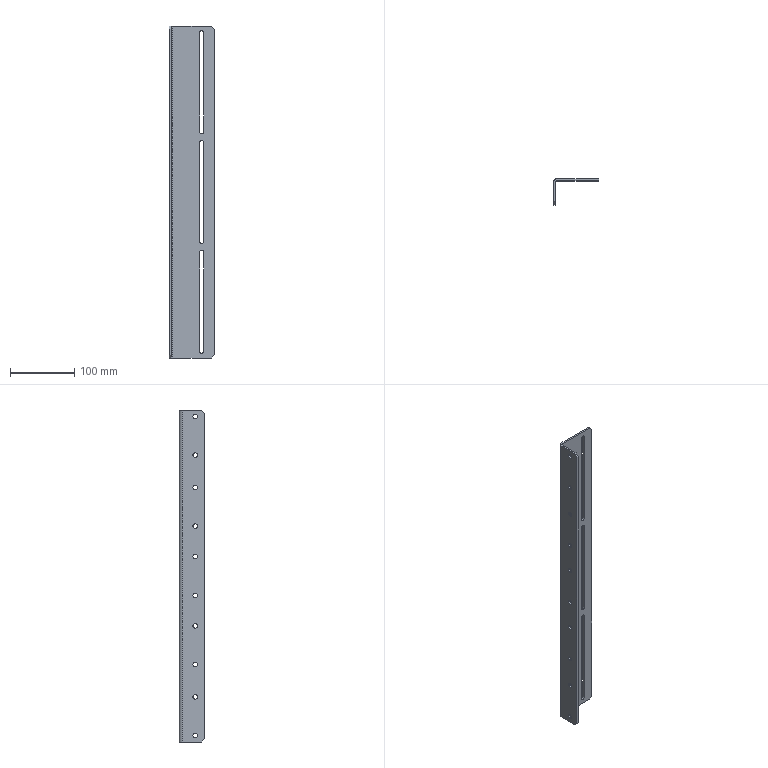Part | SolidWorks | features ICE 2, Chamfer 1, Extrusion 1 | 1 solid | 46 faces | box 70 x 40 x 515 mm | volume 153119 mm3 | cylinder 28 | plane 18 | commonest cylinder face diameters 7 x20 6 x6 4 x1 10 x1
STEP:
#1=CARTESIAN_POINT('',(-67.,-25.,13.5));
#2=VERTEX_POINT('',#1);
#3=CARTESIAN_POINT('',(-67.,-25.,6.5));
#4=VERTEX_POINT('',#3);
#5=CARTESIAN_POINT('',(-67.,-25.,10.));
#6=DIRECTION('',(1.,0.,0.));
#7=DIRECTION('',(0.,0.,-1.));
#8=AXIS2_PLACEMENT_3D('',#5,#6,#7);
#9=CIRCLE('',#8,3.5);
#10=EDGE_CURVE('',#2,#4,#9,.T.);
#11=ORIENTED_EDGE('',*,*,#10,.T.);
#12=CARTESIAN_POINT('',(-70.,-25.,6.5));
#13=VERTEX_POINT('',#12);
#14=CARTESIAN_POINT('',(445.,-25.,6.5));
#15=DIRECTION('',(-1.,0.,0.));
#16=VECTOR('',#15,1000.);
#17=LINE('',#14,#16);
#18=EDGE_CURVE('',#4,#13,#17,.T.);
#19=ORIENTED_EDGE('',*,*,#18,.T.);
#20=CARTESIAN_POINT('',(-70.,-25.,13.5));
#21=VERTEX_POINT('',#20);
#22=CARTESIAN_POINT('',(-70.,-25.,10.));
#23=DIRECTION('',(-1.,0.,0.));
#24=DIRECTION('',(0.,0.,1.));
#25=AXIS2_PLACEMENT_3D('',#22,#23,#24);
#26=CIRCLE('',#25,3.5);
#27=EDGE_CURVE('',#13,#21,#26,.T.);
#28=ORIENTED_EDGE('',*,*,#27,.T.);
#29=CARTESIAN_POINT('',(445.,-25.,13.5));
#30=DIRECTION('',(-1.,0.,0.));
#31=VECTOR('',#30,1000.);
#32=LINE('',#29,#31);
#33=EDGE_CURVE('',#2,#21,#32,.T.);
#34=ORIENTED_EDGE('',*,*,#33,.F.);
#35=EDGE_LOOP('',(#11,#19,#28,#34));
#36=FACE_OUTER_BOUND('',#35,.T.);
#37=CARTESIAN_POINT('',(445.,-25.,10.));
#38=DIRECTION('',(-1.,0.,0.));
#39=DIRECTION('',(0.,0.,1.));
#40=AXIS2_PLACEMENT_3D('',#37,#38,#39);
#41=CYLINDRICAL_SURFACE('',#40,3.5);
#42=ADVANCED_FACE('',(#36),#41,.F.);
#43=CARTESIAN_POINT('',(-67.,-25.,338.5));
#44=VERTEX_POINT('',#43);
#45=CARTESIAN_POINT('',(-67.,-25.,331.5));
#46=VERTEX_POINT('',#45);
#47=CARTESIAN_POINT('',(-67.,-25.,335.));
#48=DIRECTION('',(1.,0.,0.));
#49=DIRECTION('',(0.,0.,-1.));
#50=AXIS2_PLACEMENT_3D('',#47,#48,#49);
#51=CIRCLE('',#50,3.5);
#52=EDGE_CURVE('',#44,#46,#51,.T.);
#53=ORIENTED_EDGE('',*,*,#52,.T.);
#54=CARTESIAN_POINT('',(-70.,-25.,331.5));
#55=VERTEX_POINT('',#54);
#56=CARTESIAN_POINT('',(445.,-25.,331.5));
#57=DIRECTION('',(-1.,0.,0.));
#58=VECTOR('',#57,1000.);
#59=LINE('',#56,#58);
#60=EDGE_CURVE('',#46,#55,#59,.T.);
#61=ORIENTED_EDGE('',*,*,#60,.T.);
#62=CARTESIAN_POINT('',(-70.,-25.,338.5));
#63=VERTEX_POINT('',#62);
#64=CARTESIAN_POINT('',(-70.,-25.,335.));
#65=DIRECTION('',(-1.,0.,0.));
#66=DIRECTION('',(0.,0.,-1.));
#67=AXIS2_PLACEMENT_3D('',#64,#65,#66);
#68=CIRCLE('',#67,3.5);
#69=EDGE_CURVE('',#55,#63,#68,.T.);
#70=ORIENTED_EDGE('',*,*,#69,.T.);
#71=CARTESIAN_POINT('',(445.,-25.,338.5));
#72=DIRECTION('',(-1.,0.,0.));
#73=VECTOR('',#72,1000.);
#74=LINE('',#71,#73);
#75=EDGE_CURVE('',#44,#63,#74,.T.);
#76=ORIENTED_EDGE('',*,*,#75,.F.);
#77=EDGE_LOOP('',(#53,#61,#70,#76));
#78=FACE_OUTER_BOUND('',#77,.T.);
#79=CARTESIAN_POINT('',(445.,-25.,335.));
#80=DIRECTION('',(-1.,0.,0.));
#81=DIRECTION('',(0.,0.,1.));
#82=AXIS2_PLACEMENT_3D('',#79,#80,#81);
#83=CYLINDRICAL_SURFACE('',#82,3.5);
#84=ADVANCED_FACE('',(#78),#83,.F.);
#85=CARTESIAN_POINT('',(-67.,-25.,183.5));
#86=VERTEX_POINT('',#85);
#87=CARTESIAN_POINT('',(-67.,-25.,176.5));
#88=VERTEX_POINT('',#87);
#89=CARTESIAN_POINT('',(-67.,-25.,180.));
#90=DIRECTION('',(1.,0.,0.));
#91=DIRECTION('',(0.,0.,-1.));
#92=AXIS2_PLACEMENT_3D('',#89,#90,#91);
#93=CIRCLE('',#92,3.5);
#94=EDGE_CURVE('',#86,#88,#93,.T.);
#95=ORIENTED_EDGE('',*,*,#94,.T.);
#96=CARTESIAN_POINT('',(-70.,-25.,176.5));
#97=VERTEX_POINT('',#96);
#98=CARTESIAN_POINT('',(445.,-25.,176.5));
#99=DIRECTION('',(-1.,0.,0.));
#100=VECTOR('',#99,1000.);
#101=LINE('',#98,#100);
#102=EDGE_CURVE('',#88,#97,#101,.T.);
#103=ORIENTED_EDGE('',*,*,#102,.T.);
#104=CARTESIAN_POINT('',(-70.,-25.,183.5));
#105=VERTEX_POINT('',#104);
#106=CARTESIAN_POINT('',(-70.,-25.,180.));
#107=DIRECTION('',(-1.,0.,0.));
#108=DIRECTION('',(0.,0.,1.));
#109=AXIS2_PLACEMENT_3D('',#106,#107,#108);
#110=CIRCLE('',#109,3.5);
#111=EDGE_CURVE('',#97,#105,#110,.T.);
#112=ORIENTED_EDGE('',*,*,#111,.T.);
#113=CARTESIAN_POINT('',(445.,-25.,183.5));
#114=DIRECTION('',(-1.,0.,0.));
#115=VECTOR('',#114,1000.);
#116=LINE('',#113,#115);
#117=EDGE_CURVE('',#86,#105,#116,.T.);
#118=ORIENTED_EDGE('',*,*,#117,.F.);
#119=EDGE_LOOP('',(#95,#103,#112,#118));
#120=FACE_OUTER_BOUND('',#119,.T.);
#121=CARTESIAN_POINT('',(445.,-25.,180.));
#122=DIRECTION('',(-1.,0.,0.));
#123=DIRECTION('',(0.,0.,1.));
#124=AXIS2_PLACEMENT_3D('',#121,#122,#123);
#125=CYLINDRICAL_SURFACE('',#124,3.5);
#126=ADVANCED_FACE('',(#120),#125,.F.);
#127=CARTESIAN_POINT('',(-67.,-25.,291.));
#128=VERTEX_POINT('',#127);
#129=CARTESIAN_POINT('',(-67.,-25.,284.));
#130=VERTEX_POINT('',#129);
#131=CARTESIAN_POINT('',(-67.,-25.,287.5));
#132=DIRECTION('',(1.,0.,0.));
#133=DIRECTION('',(0.,0.,-1.));
#134=AXIS2_PLACEMENT_3D('',#131,#132,#133);
#135=CIRCLE('',#134,3.5);
#136=EDGE_CURVE('',#128,#130,#135,.T.);
#137=ORIENTED_EDGE('',*,*,#136,.T.);
#138=CARTESIAN_POINT('',(-70.,-25.,284.));
#139=VERTEX_POINT('',#138);
#140=CARTESIAN_POINT('',(445.,-25.,284.));
#141=DIRECTION('',(-1.,0.,0.));
#142=VECTOR('',#141,1000.);
#143=LINE('',#140,#142);
#144=EDGE_CURVE('',#130,#139,#143,.T.);
#145=ORIENTED_EDGE('',*,*,#144,.T.);
#146=CARTESIAN_POINT('',(-70.,-25.,291.));
#147=VERTEX_POINT('',#146);
#148=CARTESIAN_POINT('',(-70.,-25.,287.5));
#149=DIRECTION('',(-1.,0.,0.));
#150=DIRECTION('',(0.,0.,1.));
#151=AXIS2_PLACEMENT_3D('',#148,#149,#150);
#152=CIRCLE('',#151,3.5);
#153=EDGE_CURVE('',#139,#147,#152,.T.);
#154=ORIENTED_EDGE('',*,*,#153,.T.);
#155=CARTESIAN_POINT('',(445.,-25.,291.));
#156=DIRECTION('',(-1.,0.,0.));
#157=VECTOR('',#156,1000.);
#158=LINE('',#155,#157);
#159=EDGE_CURVE('',#128,#147,#158,.T.);
#160=ORIENTED_EDGE('',*,*,#159,.F.);
#161=EDGE_LOOP('',(#137,#145,#154,#160));
#162=FACE_OUTER_BOUND('',#161,.T.);
#163=CARTESIAN_POINT('',(445.,-25.,287.5));
#164=DIRECTION('',(-1.,0.,0.));
#165=DIRECTION('',(0.,0.,1.));
#166=AXIS2_PLACEMENT_3D('',#163,#164,#165);
#167=CYLINDRICAL_SURFACE('',#166,3.5);
#168=ADVANCED_FACE('',(#162),#167,.F.);
#169=CARTESIAN_POINT('',(-67.,-25.,448.5));
#170=VERTEX_POINT('',#169);
#171=CARTESIAN_POINT('',(-67.,-25.,441.5));
#172=VERTEX_POINT('',#171);
#173=CARTESIAN_POINT('',(-67.,-25.,445.));
#174=DIRECTION('',(1.,0.,0.));
#175=DIRECTION('',(0.,0.,-1.));
#176=AXIS2_PLACEMENT_3D('',#173,#174,#175);
#177=CIRCLE('',#176,3.5);
#178=EDGE_CURVE('',#170,#172,#177,.T.);
#179=ORIENTED_EDGE('',*,*,#178,.T.);
#180=CARTESIAN_POINT('',(-70.,-25.,441.5));
#181=VERTEX_POINT('',#180);
#182=CARTESIAN_POINT('',(445.,-25.,441.5));
#183=DIRECTION('',(-1.,0.,0.));
#184=VECTOR('',#183,1000.);
#185=LINE('',#182,#184);
#186=EDGE_CURVE('',#172,#181,#185,.T.);
#187=ORIENTED_EDGE('',*,*,#186,.T.);
#188=CARTESIAN_POINT('',(-70.,-25.,448.5));
#189=VERTEX_POINT('',#188);
#190=CARTESIAN_POINT('',(-70.,-25.,445.));
#191=DIRECTION('',(-1.,0.,0.));
#192=DIRECTION('',(0.,0.,-1.));
#193=AXIS2_PLACEMENT_3D('',#190,#191,#192);
#194=CIRCLE('',#193,3.5);
#195=EDGE_CURVE('',#181,#189,#194,.T.);
#196=ORIENTED_EDGE('',*,*,#195,.T.);
#197=CARTESIAN_POINT('',(445.,-25.,448.5));
#198=DIRECTION('',(-1.,0.,0.));
#199=VECTOR('',#198,1000.);
#200=LINE('',#197,#199);
#201=EDGE_CURVE('',#170,#189,#200,.T.);
#202=ORIENTED_EDGE('',*,*,#201,.F.);
#203=EDGE_LOOP('',(#179,#187,#196,#202));
#204=FACE_OUTER_BOUND('',#203,.T.);
#205=CARTESIAN_POINT('',(445.,-25.,445.));
#206=DIRECTION('',(-1.,0.,0.));
#207=DIRECTION('',(0.,0.,1.));
#208=AXIS2_PLACEMENT_3D('',#205,#206,#207);
#209=CYLINDRICAL_SURFACE('',#208,3.5);
#210=ADVANCED_FACE('',(#204),#209,.F.);
#211=CARTESIAN_POINT('',(-67.,-25.,73.5));
#212=VERTEX_POINT('',#211);
#213=CARTESIAN_POINT('',(-67.,-25.,66.5));
#214=VERTEX_POINT('',#213);
#215=CARTESIAN_POINT('',(-67.,-25.,70.));
#216=DIRECTION('',(1.,0.,0.));
#217=DIRECTION('',(0.,0.,-1.));
#218=AXIS2_PLACEMENT_3D('',#215,#216,#217);
#219=CIRCLE('',#218,3.5);
#220=EDGE_CURVE('',#212,#214,#219,.T.);
#221=ORIENTED_EDGE('',*,*,#220,.T.);
#222=CARTESIAN_POINT('',(-70.,-25.,66.5));
#223=VERTEX_POINT('',#222);
#224=CARTESIAN_POINT('',(445.,-25.,66.5));
#225=DIRECTION('',(-1.,0.,0.));
#226=VECTOR('',#225,1000.);
#227=LINE('',#224,#226);
#228=EDGE_CURVE('',#214,#223,#227,.T.);
#229=ORIENTED_EDGE('',*,*,#228,.T.);
#230=CARTESIAN_POINT('',(-70.,-25.,73.5));
#231=VERTEX_POINT('',#230);
#232=CARTESIAN_POINT('',(-70.,-25.,70.));
#233=DIRECTION('',(-1.,0.,0.));
#234=DIRECTION('',(0.,0.,1.));
#235=AXIS2_PLACEMENT_3D('',#232,#233,#234);
#236=CIRCLE('',#235,3.5);
#237=EDGE_CURVE('',#223,#231,#236,.T.);
#238=ORIENTED_EDGE('',*,*,#237,.T.);
#239=CARTESIAN_POINT('',(445.,-25.,73.5));
#240=DIRECTION('',(-1.,0.,0.));
#241=VECTOR('',#240,1000.);
#242=LINE('',#239,#241);
#243=EDGE_CURVE('',#212,#231,#242,.T.);
#244=ORIENTED_EDGE('',*,*,#243,.F.);
#245=EDGE_LOOP('',(#221,#229,#238,#244));
#246=FACE_OUTER_BOUND('',#245,.T.);
#247=CARTESIAN_POINT('',(445.,-25.,70.));
#248=DIRECTION('',(-1.,0.,0.));
#249=DIRECTION('',(0.,0.,1.));
#250=AXIS2_PLACEMENT_3D('',#247,#248,#249);
#251=CYLINDRICAL_SURFACE('',#250,3.5);
#252=ADVANCED_FACE('',(#246),#251,.F.);
#253=CARTESIAN_POINT('',(-67.,-25.,123.5));
#254=VERTEX_POINT('',#253);
#255=CARTESIAN_POINT('',(-67.,-25.,116.5));
#256=VERTEX_POINT('',#255);
#257=CARTESIAN_POINT('',(-67.,-25.,120.));
#258=DIRECTION('',(1.,0.,0.));
#259=DIRECTION('',(0.,0.,-1.));
#260=AXIS2_PLACEMENT_3D('',#257,#258,#259);
#261=CIRCLE('',#260,3.5);
#262=EDGE_CURVE('',#254,#256,#261,.T.);
#263=ORIENTED_EDGE('',*,*,#262,.T.);
#264=CARTESIAN_POINT('',(-70.,-25.,116.5));
#265=VERTEX_POINT('',#264);
#266=CARTESIAN_POINT('',(445.,-25.,116.5));
#267=DIRECTION('',(-1.,0.,0.));
#268=VECTOR('',#267,1000.);
#269=LINE('',#266,#268);
#270=EDGE_CURVE('',#256,#265,#269,.T.);
#271=ORIENTED_EDGE('',*,*,#270,.T.);
#272=CARTESIAN_POINT('',(-70.,-25.,123.5));
#273=VERTEX_POINT('',#272);
#274=CARTESIAN_POINT('',(-70.,-25.,120.));
#275=DIRECTION('',(-1.,0.,0.));
#276=DIRECTION('',(0.,0.,1.));
#277=AXIS2_PLACEMENT_3D('',#274,#275,#276);
#278=CIRCLE('',#277,3.5);
#279=EDGE_CURVE('',#265,#273,#278,.T.);
#280=ORIENTED_EDGE('',*,*,#279,.T.);
#281=CARTESIAN_POINT('',(445.,-25.,123.5));
#282=DIRECTION('',(-1.,0.,0.));
#283=VECTOR('',#282,1000.);
#284=LINE('',#281,#283);
#285=EDGE_CURVE('',#254,#273,#284,.T.);
#286=ORIENTED_EDGE('',*,*,#285,.F.);
#287=EDGE_LOOP('',(#263,#271,#280,#286));
#288=FACE_OUTER_BOUND('',#287,.T.);
#289=CARTESIAN_POINT('',(445.,-25.,120.));
#290=DIRECTION('',(-1.,0.,0.));
#291=DIRECTION('',(0.,0.,1.));
#292=AXIS2_PLACEMENT_3D('',#289,#290,#291);
#293=CYLINDRICAL_SURFACE('',#292,3.5);
#294=ADVANCED_FACE('',(#288),#293,.F.);
#295=CARTESIAN_POINT('',(-67.,-25.,231.));
#296=VERTEX_POINT('',#295);
#297=CARTESIAN_POINT('',(-67.,-25.,224.));
#298=VERTEX_POINT('',#297);
#299=CARTESIAN_POINT('',(-67.,-25.,227.5));
#300=DIRECTION('',(1.,0.,0.));
#301=DIRECTION('',(0.,0.,-1.));
#302=AXIS2_PLACEMENT_3D('',#299,#300,#301);
#303=CIRCLE('',#302,3.5);
#304=EDGE_CURVE('',#296,#298,#303,.T.);
#305=ORIENTED_EDGE('',*,*,#304,.T.);
#306=CARTESIAN_POINT('',(-70.,-25.,224.));
#307=VERTEX_POINT('',#306);
#308=CARTESIAN_POINT('',(445.,-25.,224.));
#309=DIRECTION('',(-1.,0.,0.));
#310=VECTOR('',#309,1000.);
#311=LINE('',#308,#310);
#312=EDGE_CURVE('',#298,#307,#311,.T.);
#313=ORIENTED_EDGE('',*,*,#312,.T.);
#314=CARTESIAN_POINT('',(-70.,-25.,231.));
#315=VERTEX_POINT('',#314);
#316=CARTESIAN_POINT('',(-70.,-25.,227.5));
#317=DIRECTION('',(-1.,0.,0.));
#318=DIRECTION('',(0.,0.,1.));
#319=AXIS2_PLACEMENT_3D('',#316,#317,#318);
#320=CIRCLE('',#319,3.5);
#321=EDGE_CURVE('',#307,#315,#320,.T.);
#322=ORIENTED_EDGE('',*,*,#321,.T.);
#323=CARTESIAN_POINT('',(445.,-25.,231.));
#324=DIRECTION('',(-1.,0.,0.));
#325=VECTOR('',#324,1000.);
#326=LINE('',#323,#325);
#327=EDGE_CURVE('',#296,#315,#326,.T.);
#328=ORIENTED_EDGE('',*,*,#327,.F.);
#329=EDGE_LOOP('',(#305,#313,#322,#328));
#330=FACE_OUTER_BOUND('',#329,.T.);
#331=CARTESIAN_POINT('',(445.,-25.,227.5));
#332=DIRECTION('',(-1.,0.,0.));
#333=DIRECTION('',(0.,0.,1.));
#334=AXIS2_PLACEMENT_3D('',#331,#332,#333);
#335=CYLINDRICAL_SURFACE('',#334,3.5);
#336=ADVANCED_FACE('',(#330),#335,.F.);
#337=CARTESIAN_POINT('',(-67.,-25.,508.5));
#338=VERTEX_POINT('',#337);
#339=CARTESIAN_POINT('',(-67.,-25.,501.5));
#340=VERTEX_POINT('',#339);
#341=CARTESIAN_POINT('',(-67.,-25.,505.));
#342=DIRECTION('',(1.,0.,0.));
#343=DIRECTION('',(0.,0.,-1.));
#344=AXIS2_PLACEMENT_3D('',#341,#342,#343);
#345=CIRCLE('',#344,3.5);
#346=EDGE_CURVE('',#338,#340,#345,.T.);
#347=ORIENTED_EDGE('',*,*,#346,.T.);
#348=CARTESIAN_POINT('',(-70.,-25.,501.5));
#349=VERTEX_POINT('',#348);
#350=CARTESIAN_POINT('',(445.,-25.,501.5));
#351=DIRECTION('',(-1.,0.,0.));
#352=VECTOR('',#351,1000.);
#353=LINE('',#350,#352);
#354=EDGE_CURVE('',#340,#349,#353,.T.);
#355=ORIENTED_EDGE('',*,*,#354,.T.);
#356=CARTESIAN_POINT('',(-70.,-25.,508.5));
#357=VERTEX_POINT('',#356);
#358=CARTESIAN_POINT('',(-70.,-25.,505.));
#359=DIRECTION('',(-1.,0.,0.));
#360=DIRECTION('',(0.,0.,-1.));
#361=AXIS2_PLACEMENT_3D('',#358,#359,#360);
#362=CIRCLE('',#361,3.5);
#363=EDGE_CURVE('',#349,#357,#362,.T.);
#364=ORIENTED_EDGE('',*,*,#363,.T.);
#365=CARTESIAN_POINT('',(445.,-25.,508.5));
#366=DIRECTION('',(-1.,0.,0.));
#367=VECTOR('',#366,1000.);
#368=LINE('',#365,#367);
#369=EDGE_CURVE('',#338,#357,#368,.T.);
#370=ORIENTED_EDGE('',*,*,#369,.F.);
#371=EDGE_LOOP('',(#347,#355,#364,#370));
#372=FACE_OUTER_BOUND('',#371,.T.);
#373=CARTESIAN_POINT('',(445.,-25.,505.));
#374=DIRECTION('',(-1.,0.,0.));
#375=DIRECTION('',(0.,0.,1.));
#376=AXIS2_PLACEMENT_3D('',#373,#374,#375);
#377=CYLINDRICAL_SURFACE('',#376,3.5);
#378=ADVANCED_FACE('',(#372),#377,.F.);
#379=CARTESIAN_POINT('',(-67.,-25.,398.5));
#380=VERTEX_POINT('',#379);
#381=CARTESIAN_POINT('',(-67.,-25.,391.5));
#382=VERTEX_POINT('',#381);
#383=CARTESIAN_POINT('',(-67.,-25.,395.));
#384=DIRECTION('',(1.,0.,0.));
#385=DIRECTION('',(0.,0.,-1.));
#386=AXIS2_PLACEMENT_3D('',#383,#384,#385);
#387=CIRCLE('',#386,3.5);
#388=EDGE_CURVE('',#380,#382,#387,.T.);
#389=ORIENTED_EDGE('',*,*,#388,.T.);
#390=CARTESIAN_POINT('',(-70.,-25.,391.5));
#391=VERTEX_POINT('',#390);
#392=CARTESIAN_POINT('',(445.,-25.,391.5));
#393=DIRECTION('',(-1.,0.,0.));
#394=VECTOR('',#393,1000.);
#395=LINE('',#392,#394);
#396=EDGE_CURVE('',#382,#391,#395,.T.);
#397=ORIENTED_EDGE('',*,*,#396,.T.);
#398=CARTESIAN_POINT('',(-70.,-25.,398.5));
#399=VERTEX_POINT('',#398);
#400=CARTESIAN_POINT('',(-70.,-25.,395.));
#401=DIRECTION('',(-1.,0.,0.));
#402=DIRECTION('',(0.,0.,-1.));
#403=AXIS2_PLACEMENT_3D('',#400,#401,#402);
#404=CIRCLE('',#403,3.5);
#405=EDGE_CURVE('',#391,#399,#404,.T.);
#406=ORIENTED_EDGE('',*,*,#405,.T.);
#407=CARTESIAN_POINT('',(445.,-25.,398.5));
#408=DIRECTION('',(-1.,0.,0.));
#409=VECTOR('',#408,1000.);
#410=LINE('',#407,#409);
#411=EDGE_CURVE('',#380,#399,#410,.T.);
#412=ORIENTED_EDGE('',*,*,#411,.F.);
#413=EDGE_LOOP('',(#389,#397,#406,#412));
#414=FACE_OUTER_BOUND('',#413,.T.);
#415=CARTESIAN_POINT('',(445.,-25.,395.));
#416=DIRECTION('',(-1.,0.,0.));
#417=DIRECTION('',(0.,0.,1.));
#418=AXIS2_PLACEMENT_3D('',#415,#416,#417);
#419=CYLINDRICAL_SURFACE('',#418,3.5);
#420=ADVANCED_FACE('',(#414),#419,.F.);
#421=CARTESIAN_POINT('',(-70.,-25.,10.));
#422=DIRECTION('',(-1.,0.,0.));
#423=DIRECTION('',(0.,0.,1.));
#424=AXIS2_PLACEMENT_3D('',#421,#422,#423);
#425=CIRCLE('',#424,3.5);
#426=EDGE_CURVE('',#21,#13,#425,.T.);
#427=ORIENTED_EDGE('',*,*,#426,.F.);
#428=ORIENTED_EDGE('',*,*,#27,.F.);
#429=EDGE_LOOP('',(#427,#428));
#430=FACE_BOUND('',#429,.T.);
#431=CARTESIAN_POINT('',(-70.,-25.,335.));
#432=DIRECTION('',(-1.,0.,0.));
#433=DIRECTION('',(0.,0.,-1.));
#434=AXIS2_PLACEMENT_3D('',#431,#432,#433);
#435=CIRCLE('',#434,3.5);
#436=EDGE_CURVE('',#63,#55,#435,.T.);
#437=ORIENTED_EDGE('',*,*,#436,.F.);
#438=ORIENTED_EDGE('',*,*,#69,.F.);
#439=EDGE_LOOP('',(#437,#438));
#440=FACE_BOUND('',#439,.T.);
#441=CARTESIAN_POINT('',(-70.,-25.,180.));
#442=DIRECTION('',(-1.,0.,0.));
#443=DIRECTION('',(0.,0.,1.));
#444=AXIS2_PLACEMENT_3D('',#441,#442,#443);
#445=CIRCLE('',#444,3.5);
#446=EDGE_CURVE('',#105,#97,#445,.T.);
#447=ORIENTED_EDGE('',*,*,#446,.F.);
#448=ORIENTED_EDGE('',*,*,#111,.F.);
#449=EDGE_LOOP('',(#447,#448));
#450=FACE_BOUND('',#449,.T.);
#451=CARTESIAN_POINT('',(-70.,-25.,287.5));
#452=DIRECTION('',(-1.,0.,0.));
#453=DIRECTION('',(0.,0.,1.));
#454=AXIS2_PLACEMENT_3D('',#451,#452,#453);
#455=CIRCLE('',#454,3.5);
#456=EDGE_CURVE('',#147,#139,#455,.T.);
#457=ORIENTED_EDGE('',*,*,#456,.F.);
#458=ORIENTED_EDGE('',*,*,#153,.F.);
#459=EDGE_LOOP('',(#457,#458));
#460=FACE_BOUND('',#459,.T.);
#461=CARTESIAN_POINT('',(-70.,-25.,445.));
#462=DIRECTION('',(-1.,0.,0.));
#463=DIRECTION('',(0.,0.,-1.));
#464=AXIS2_PLACEMENT_3D('',#461,#462,#463);
#465=CIRCLE('',#464,3.5);
#466=EDGE_CURVE('',#189,#181,#465,.T.);
#467=ORIENTED_EDGE('',*,*,#466,.F.);
#468=ORIENTED_EDGE('',*,*,#195,.F.);
#469=EDGE_LOOP('',(#467,#468));
#470=FACE_BOUND('',#469,.T.);
#471=CARTESIAN_POINT('',(-70.,-25.,70.));
#472=DIRECTION('',(-1.,0.,0.));
#473=DIRECTION('',(0.,0.,1.));
#474=AXIS2_PLACEMENT_3D('',#471,#472,#473);
#475=CIRCLE('',#474,3.5);
#476=EDGE_CURVE('',#231,#223,#475,.T.);
#477=ORIENTED_EDGE('',*,*,#476,.F.);
#478=ORIENTED_EDGE('',*,*,#237,.F.);
#479=EDGE_LOOP('',(#477,#478));
#480=FACE_BOUND('',#479,.T.);
#481=CARTESIAN_POINT('',(-70.,-25.,120.));
#482=DIRECTION('',(-1.,0.,0.));
#483=DIRECTION('',(0.,0.,1.));
#484=AXIS2_PLACEMENT_3D('',#481,#482,#483);
#485=CIRCLE('',#484,3.5);
#486=EDGE_CURVE('',#273,#265,#485,.T.);
#487=ORIENTED_EDGE('',*,*,#486,.F.);
#488=ORIENTED_EDGE('',*,*,#279,.F.);
#489=EDGE_LOOP('',(#487,#488));
#490=FACE_BOUND('',#489,.T.);
#491=CARTESIAN_POINT('',(-70.,-25.,227.5));
#492=DIRECTION('',(-1.,0.,0.));
#493=DIRECTION('',(0.,0.,1.));
#494=AXIS2_PLACEMENT_3D('',#491,#492,#493);
#495=CIRCLE('',#494,3.5);
#496=EDGE_CURVE('',#315,#307,#495,.T.);
#497=ORIENTED_EDGE('',*,*,#496,.F.);
#498=ORIENTED_EDGE('',*,*,#321,.F.);
#499=EDGE_LOOP('',(#497,#498));
#500=FACE_BOUND('',#499,.T.);
#501=CARTESIAN_POINT('',(-70.,-25.,505.));
#502=DIRECTION('',(-1.,0.,0.));
#503=DIRECTION('',(0.,0.,-1.));
#504=AXIS2_PLACEMENT_3D('',#501,#502,#503);
#505=CIRCLE('',#504,3.5);
#506=EDGE_CURVE('',#357,#349,#505,.T.);
#507=ORIENTED_EDGE('',*,*,#506,.F.);
#508=ORIENTED_EDGE('',*,*,#363,.F.);
#509=EDGE_LOOP('',(#507,#508));
#510=FACE_BOUND('',#509,.T.);
#511=CARTESIAN_POINT('',(-70.,-25.,395.));
#512=DIRECTION('',(-1.,0.,0.));
#513=DIRECTION('',(0.,0.,-1.));
#514=AXIS2_PLACEMENT_3D('',#511,#512,#513);
#515=CIRCLE('',#514,3.5);
#516=EDGE_CURVE('',#399,#391,#515,.T.);
#517=ORIENTED_EDGE('',*,*,#516,.F.);
#518=ORIENTED_EDGE('',*,*,#405,.F.);
#519=EDGE_LOOP('',(#517,#518));
#520=FACE_BOUND('',#519,.T.);
#521=CARTESIAN_POINT('',(-70.,-40.,510.));
#522=VERTEX_POINT('',#521);
#523=CARTESIAN_POINT('',(-70.,-40.,5.));
#524=VERTEX_POINT('',#523);
#525=CARTESIAN_POINT('',(-70.,-40.,515.));
#526=DIRECTION('',(0.,0.,-1.));
#527=VECTOR('',#526,1000.);
#528=LINE('',#525,#527);
#529=EDGE_CURVE('',#522,#524,#528,.T.);
#530=ORIENTED_EDGE('',*,*,#529,.F.);
#531=CARTESIAN_POINT('',(-70.,-35.,515.));
#532=VERTEX_POINT('',#531);
#533=CARTESIAN_POINT('',(-70.,-35.,515.));
#534=DIRECTION('',(0.,0.7071,0.7071));
#535=VECTOR('',#534,1000.);
#536=LINE('',#533,#535);
#537=EDGE_CURVE('',#522,#532,#536,.T.);
#538=ORIENTED_EDGE('',*,*,#537,.T.);
#539=CARTESIAN_POINT('',(-70.,-5.,515.));
#540=VERTEX_POINT('',#539);
#541=CARTESIAN_POINT('',(-70.,-5.,515.));
#542=DIRECTION('',(0.,-1.,0.));
#543=VECTOR('',#542,1000.);
#544=LINE('',#541,#543);
#545=EDGE_CURVE('',#540,#532,#544,.T.);
#546=ORIENTED_EDGE('',*,*,#545,.F.);
#547=CARTESIAN_POINT('',(-70.,-5.,0.));
#548=VERTEX_POINT('',#547);
#549=CARTESIAN_POINT('',(-70.,-5.,515.));
#550=DIRECTION('',(0.,0.,-1.));
#551=VECTOR('',#550,1000.);
#552=LINE('',#549,#551);
#553=EDGE_CURVE('',#540,#548,#552,.T.);
#554=ORIENTED_EDGE('',*,*,#553,.T.);
#555=CARTESIAN_POINT('',(-70.,-35.,0.));
#556=VERTEX_POINT('',#555);
#557=CARTESIAN_POINT('',(-70.,-5.,0.));
#558=DIRECTION('',(0.,-1.,0.));
#559=VECTOR('',#558,1000.);
#560=LINE('',#557,#559);
#561=EDGE_CURVE('',#548,#556,#560,.T.);
#562=ORIENTED_EDGE('',*,*,#561,.T.);
#563=CARTESIAN_POINT('',(-70.,-40.,5.));
#564=DIRECTION('',(0.,-0.7071,0.7071));
#565=VECTOR('',#564,1000.);
#566=LINE('',#563,#565);
#567=EDGE_CURVE('',#556,#524,#566,.T.);
#568=ORIENTED_EDGE('',*,*,#567,.T.);
#569=EDGE_LOOP('',(#530,#538,#546,#554,#562,#568));
#570=FACE_OUTER_BOUND('',#569,.T.);
#571=CARTESIAN_POINT('',(-70.,-5.,515.));
#572=DIRECTION('',(1.,0.,0.));
#573=DIRECTION('',(0.,0.,-1.));
#574=AXIS2_PLACEMENT_3D('',#571,#572,#573);
#575=PLANE('',#574);
#576=ADVANCED_FACE('',(#430,#440,#450,#460,#470,#480,#490,#500,#510,#520,#570),#575,.F.);
#577=CARTESIAN_POINT('',(-67.,-40.,510.));
#578=VERTEX_POINT('',#577);
#579=CARTESIAN_POINT('',(-67.,-40.,5.));
#580=VERTEX_POINT('',#579);
#581=CARTESIAN_POINT('',(-67.,-40.,515.));
#582=DIRECTION('',(0.,0.,-1.));
#583=VECTOR('',#582,1000.);
#584=LINE('',#581,#583);
#585=EDGE_CURVE('',#578,#580,#584,.T.);
#586=ORIENTED_EDGE('',*,*,#585,.F.);
#587=CARTESIAN_POINT('',(-70.,-40.,510.));
#588=DIRECTION('',(-1.,0.,0.));
#589=VECTOR('',#588,1000.);
#590=LINE('',#587,#589);
#591=EDGE_CURVE('',#578,#522,#590,.T.);
#592=ORIENTED_EDGE('',*,*,#591,.T.);
#593=ORIENTED_EDGE('',*,*,#529,.T.);
#594=CARTESIAN_POINT('',(-70.,-40.,5.));
#595=DIRECTION('',(1.,0.,0.));
#596=VECTOR('',#595,1000.);
#597=LINE('',#594,#596);
#598=EDGE_CURVE('',#524,#580,#597,.T.);
#599=ORIENTED_EDGE('',*,*,#598,.T.);
#600=EDGE_LOOP('',(#586,#592,#593,#599));
#601=FACE_OUTER_BOUND('',#600,.T.);
#602=CARTESIAN_POINT('',(-70.,-40.,515.));
#603=DIRECTION('',(0.,1.,0.));
#604=DIRECTION('',(0.,0.,1.));
#605=AXIS2_PLACEMENT_3D('',#602,#603,#604);
#606=PLANE('',#605);
#607=ADVANCED_FACE('',(#601),#606,.F.);
#608=ORIENTED_EDGE('',*,*,#10,.F.);
#609=CARTESIAN_POINT('',(-67.,-25.,10.));
#610=DIRECTION('',(1.,0.,0.));
#611=DIRECTION('',(0.,0.,-1.));
#612=AXIS2_PLACEMENT_3D('',#609,#610,#611);
#613=CIRCLE('',#612,3.5);
#614=EDGE_CURVE('',#4,#2,#613,.T.);
#615=ORIENTED_EDGE('',*,*,#614,.F.);
#616=EDGE_LOOP('',(#608,#615));
#617=FACE_BOUND('',#616,.T.);
#618=ORIENTED_EDGE('',*,*,#52,.F.);
#619=CARTESIAN_POINT('',(-67.,-25.,335.));
#620=DIRECTION('',(1.,0.,0.));
#621=DIRECTION('',(0.,0.,-1.));
#622=AXIS2_PLACEMENT_3D('',#619,#620,#621);
#623=CIRCLE('',#622,3.5);
#624=EDGE_CURVE('',#46,#44,#623,.T.);
#625=ORIENTED_EDGE('',*,*,#624,.F.);
#626=EDGE_LOOP('',(#618,#625));
#627=FACE_BOUND('',#626,.T.);
#628=ORIENTED_EDGE('',*,*,#94,.F.);
#629=CARTESIAN_POINT('',(-67.,-25.,180.));
#630=DIRECTION('',(1.,0.,0.));
#631=DIRECTION('',(0.,0.,-1.));
#632=AXIS2_PLACEMENT_3D('',#629,#630,#631);
#633=CIRCLE('',#632,3.5);
#634=EDGE_CURVE('',#88,#86,#633,.T.);
#635=ORIENTED_EDGE('',*,*,#634,.F.);
#636=EDGE_LOOP('',(#628,#635));
#637=FACE_BOUND('',#636,.T.);
#638=ORIENTED_EDGE('',*,*,#136,.F.);
#639=CARTESIAN_POINT('',(-67.,-25.,287.5));
#640=DIRECTION('',(1.,0.,0.));
#641=DIRECTION('',(0.,0.,-1.));
#642=AXIS2_PLACEMENT_3D('',#639,#640,#641);
#643=CIRCLE('',#642,3.5);
#644=EDGE_CURVE('',#130,#128,#643,.T.);
#645=ORIENTED_EDGE('',*,*,#644,.F.);
#646=EDGE_LOOP('',(#638,#645));
#647=FACE_BOUND('',#646,.T.);
#648=ORIENTED_EDGE('',*,*,#178,.F.);
#649=CARTESIAN_POINT('',(-67.,-25.,445.));
#650=DIRECTION('',(1.,0.,0.));
#651=DIRECTION('',(0.,0.,-1.));
#652=AXIS2_PLACEMENT_3D('',#649,#650,#651);
#653=CIRCLE('',#652,3.5);
#654=EDGE_CURVE('',#172,#170,#653,.T.);
#655=ORIENTED_EDGE('',*,*,#654,.F.);
#656=EDGE_LOOP('',(#648,#655));
#657=FACE_BOUND('',#656,.T.);
#658=ORIENTED_EDGE('',*,*,#220,.F.);
#659=CARTESIAN_POINT('',(-67.,-25.,70.));
#660=DIRECTION('',(1.,0.,0.));
#661=DIRECTION('',(0.,0.,-1.));
#662=AXIS2_PLACEMENT_3D('',#659,#660,#661);
#663=CIRCLE('',#662,3.5);
#664=EDGE_CURVE('',#214,#212,#663,.T.);
#665=ORIENTED_EDGE('',*,*,#664,.F.);
#666=EDGE_LOOP('',(#658,#665));
#667=FACE_BOUND('',#666,.T.);
#668=ORIENTED_EDGE('',*,*,#262,.F.);
#669=CARTESIAN_POINT('',(-67.,-25.,120.));
#670=DIRECTION('',(1.,0.,0.));
#671=DIRECTION('',(0.,0.,-1.));
#672=AXIS2_PLACEMENT_3D('',#669,#670,#671);
#673=CIRCLE('',#672,3.5);
#674=EDGE_CURVE('',#256,#254,#673,.T.);
#675=ORIENTED_EDGE('',*,*,#674,.F.);
#676=EDGE_LOOP('',(#668,#675));
#677=FACE_BOUND('',#676,.T.);
#678=ORIENTED_EDGE('',*,*,#304,.F.);
#679=CARTESIAN_POINT('',(-67.,-25.,227.5));
#680=DIRECTION('',(1.,0.,0.));
#681=DIRECTION('',(0.,0.,-1.));
#682=AXIS2_PLACEMENT_3D('',#679,#680,#681);
#683=CIRCLE('',#682,3.5);
#684=EDGE_CURVE('',#298,#296,#683,.T.);
#685=ORIENTED_EDGE('',*,*,#684,.F.);
#686=EDGE_LOOP('',(#678,#685));
#687=FACE_BOUND('',#686,.T.);
#688=ORIENTED_EDGE('',*,*,#346,.F.);
#689=CARTESIAN_POINT('',(-67.,-25.,505.));
#690=DIRECTION('',(1.,0.,0.));
#691=DIRECTION('',(0.,0.,-1.));
#692=AXIS2_PLACEMENT_3D('',#689,#690,#691);
#693=CIRCLE('',#692,3.5);
#694=EDGE_CURVE('',#340,#338,#693,.T.);
#695=ORIENTED_EDGE('',*,*,#694,.F.);
#696=EDGE_LOOP('',(#688,#695));
#697=FACE_BOUND('',#696,.T.);
#698=ORIENTED_EDGE('',*,*,#388,.F.);
#699=CARTESIAN_POINT('',(-67.,-25.,395.));
#700=DIRECTION('',(1.,0.,0.));
#701=DIRECTION('',(0.,0.,-1.));
#702=AXIS2_PLACEMENT_3D('',#699,#700,#701);
#703=CIRCLE('',#702,3.5);
#704=EDGE_CURVE('',#382,#380,#703,.T.);
#705=ORIENTED_EDGE('',*,*,#704,.F.);
#706=EDGE_LOOP('',(#698,#705));
#707=FACE_BOUND('',#706,.T.);
#708=CARTESIAN_POINT('',(-67.,-5.,515.));
#709=VERTEX_POINT('',#708);
#710=CARTESIAN_POINT('',(-67.,-35.,515.));
#711=VERTEX_POINT('',#710);
#712=CARTESIAN_POINT('',(-67.,-5.,515.));
#713=DIRECTION('',(0.,-1.,0.));
#714=VECTOR('',#713,1000.);
#715=LINE('',#712,#714);
#716=EDGE_CURVE('',#709,#711,#715,.T.);
#717=ORIENTED_EDGE('',*,*,#716,.T.);
#718=CARTESIAN_POINT('',(-67.,-20.,530.));
#719=DIRECTION('',(0.,-0.7071,-0.7071));
#720=VECTOR('',#719,1000.);
#721=LINE('',#718,#720);
#722=EDGE_CURVE('',#711,#578,#721,.T.);
#723=ORIENTED_EDGE('',*,*,#722,.T.);
#724=ORIENTED_EDGE('',*,*,#585,.T.);
#725=CARTESIAN_POINT('',(-67.,-35.,0.));
#726=VERTEX_POINT('',#725);
#727=CARTESIAN_POINT('',(-67.,-277.5,242.5));
#728=DIRECTION('',(0.,0.7071,-0.7071));
#729=VECTOR('',#728,1000.);
#730=LINE('',#727,#729);
#731=EDGE_CURVE('',#580,#726,#730,.T.);
#732=ORIENTED_EDGE('',*,*,#731,.T.);
#733=CARTESIAN_POINT('',(-67.,-5.,0.));
#734=VERTEX_POINT('',#733);
#735=CARTESIAN_POINT('',(-67.,-5.,0.));
#736=DIRECTION('',(0.,-1.,0.));
#737=VECTOR('',#736,1000.);
#738=LINE('',#735,#737);
#739=EDGE_CURVE('',#734,#726,#738,.T.);
#740=ORIENTED_EDGE('',*,*,#739,.F.);
#741=CARTESIAN_POINT('',(-67.,-5.,515.));
#742=DIRECTION('',(0.,0.,-1.));
#743=VECTOR('',#742,1000.);
#744=LINE('',#741,#743);
#745=EDGE_CURVE('',#709,#734,#744,.T.);
#746=ORIENTED_EDGE('',*,*,#745,.F.);
#747=EDGE_LOOP('',(#717,#723,#724,#732,#740,#746));
#748=FACE_OUTER_BOUND('',#747,.T.);
#749=CARTESIAN_POINT('',(-67.,-5.,515.));
#750=DIRECTION('',(1.,0.,0.));
#751=DIRECTION('',(0.,0.,-1.));
#752=AXIS2_PLACEMENT_3D('',#749,#750,#751);
#753=PLANE('',#752);
#754=ADVANCED_FACE('',(#617,#627,#637,#647,#657,#667,#677,#687,#697,#707,#748),#753,.T.);
#755=CARTESIAN_POINT('',(-65.,-3.,0.));
#756=VERTEX_POINT('',#755);
#757=CARTESIAN_POINT('',(-65.,-5.,0.));
#758=DIRECTION('',(0.,0.,1.));
#759=DIRECTION('',(1.,0.,0.));
#760=AXIS2_PLACEMENT_3D('',#757,#758,#759);
#761=CIRCLE('',#760,2.);
#762=EDGE_CURVE('',#756,#734,#761,.T.);
#763=ORIENTED_EDGE('',*,*,#762,.F.);
#764=CARTESIAN_POINT('',(-65.,-3.,515.));
#765=VERTEX_POINT('',#764);
#766=CARTESIAN_POINT('',(-65.,-3.,515.));
#767=DIRECTION('',(0.,0.,-1.));
#768=VECTOR('',#767,1000.);
#769=LINE('',#766,#768);
#770=EDGE_CURVE('',#765,#756,#769,.T.);
#771=ORIENTED_EDGE('',*,*,#770,.F.);
#772=CARTESIAN_POINT('',(-65.,-5.,515.));
#773=DIRECTION('',(0.,0.,1.));
#774=DIRECTION('',(1.,0.,0.));
#775=AXIS2_PLACEMENT_3D('',#772,#773,#774);
#776=CIRCLE('',#775,2.);
#777=EDGE_CURVE('',#765,#709,#776,.T.);
#778=ORIENTED_EDGE('',*,*,#777,.T.);
#779=ORIENTED_EDGE('',*,*,#745,.T.);
#780=EDGE_LOOP('',(#763,#771,#778,#779));
#781=FACE_OUTER_BOUND('',#780,.T.);
#782=CARTESIAN_POINT('',(-65.,-5.,515.));
#783=DIRECTION('',(0.,0.,-1.));
#784=DIRECTION('',(-1.,0.,0.));
#785=AXIS2_PLACEMENT_3D('',#782,#783,#784);
#786=CYLINDRICAL_SURFACE('',#785,2.);
#787=ADVANCED_FACE('',(#781),#786,.F.);
#788=CARTESIAN_POINT('',(-23.,-3.,10.5));
#789=VERTEX_POINT('',#788);
#790=CARTESIAN_POINT('',(-17.,-3.,10.5));
#791=VERTEX_POINT('',#790);
#792=CARTESIAN_POINT('',(-20.,-3.,10.5));
#793=DIRECTION('',(0.,-1.,0.));
#794=DIRECTION('',(1.,0.,0.));
#795=AXIS2_PLACEMENT_3D('',#792,#793,#794);
#796=CIRCLE('',#795,3.);
#797=EDGE_CURVE('',#789,#791,#796,.T.);
#798=ORIENTED_EDGE('',*,*,#797,.F.);
#799=CARTESIAN_POINT('',(-23.,-3.,164.5));
#800=VERTEX_POINT('',#799);
#801=CARTESIAN_POINT('',(-23.,-3.,515.));
#802=DIRECTION('',(0.,0.,-1.));
#803=VECTOR('',#802,1000.);
#804=LINE('',#801,#803);
#805=EDGE_CURVE('',#800,#789,#804,.T.);
#806=ORIENTED_EDGE('',*,*,#805,.F.);
#807=CARTESIAN_POINT('',(-17.,-3.,164.5));
#808=VERTEX_POINT('',#807);
#809=CARTESIAN_POINT('',(-20.,-3.,164.5));
#810=DIRECTION('',(0.,-1.,0.));
#811=DIRECTION('',(1.,0.,0.));
#812=AXIS2_PLACEMENT_3D('',#809,#810,#811);
#813=CIRCLE('',#812,3.);
#814=EDGE_CURVE('',#808,#800,#813,.T.);
#815=ORIENTED_EDGE('',*,*,#814,.F.);
#816=CARTESIAN_POINT('',(-17.,-3.,515.));
#817=DIRECTION('',(0.,0.,1.));
#818=VECTOR('',#817,1000.);
#819=LINE('',#816,#818);
#820=EDGE_CURVE('',#791,#808,#819,.T.);
#821=ORIENTED_EDGE('',*,*,#820,.F.);
#822=EDGE_LOOP('',(#798,#806,#815,#821));
#823=FACE_BOUND('',#822,.T.);
#824=CARTESIAN_POINT('',(-23.,-3.,180.5));
#825=VERTEX_POINT('',#824);
#826=CARTESIAN_POINT('',(-17.,-3.,180.5));
#827=VERTEX_POINT('',#826);
#828=CARTESIAN_POINT('',(-20.,-3.,180.5));
#829=DIRECTION('',(0.,-1.,0.));
#830=DIRECTION('',(1.,0.,0.));
#831=AXIS2_PLACEMENT_3D('',#828,#829,#830);
#832=CIRCLE('',#831,3.);
#833=EDGE_CURVE('',#825,#827,#832,.T.);
#834=ORIENTED_EDGE('',*,*,#833,.F.);
#835=CARTESIAN_POINT('',(-23.,-3.,334.5));
#836=VERTEX_POINT('',#835);
#837=CARTESIAN_POINT('',(-23.,-3.,515.));
#838=DIRECTION('',(0.,0.,-1.));
#839=VECTOR('',#838,1000.);
#840=LINE('',#837,#839);
#841=EDGE_CURVE('',#836,#825,#840,.T.);
#842=ORIENTED_EDGE('',*,*,#841,.F.);
#843=CARTESIAN_POINT('',(-17.,-3.,334.5));
#844=VERTEX_POINT('',#843);
#845=CARTESIAN_POINT('',(-20.,-3.,334.5));
#846=DIRECTION('',(0.,-1.,0.));
#847=DIRECTION('',(1.,0.,0.));
#848=AXIS2_PLACEMENT_3D('',#845,#846,#847);
#849=CIRCLE('',#848,3.);
#850=EDGE_CURVE('',#844,#836,#849,.T.);
#851=ORIENTED_EDGE('',*,*,#850,.F.);
#852=CARTESIAN_POINT('',(-17.,-3.,515.));
#853=DIRECTION('',(0.,0.,1.));
#854=VECTOR('',#853,1000.);
#855=LINE('',#852,#854);
#856=EDGE_CURVE('',#827,#844,#855,.T.);
#857=ORIENTED_EDGE('',*,*,#856,.F.);
#858=EDGE_LOOP('',(#834,#842,#851,#857));
#859=FACE_BOUND('',#858,.T.);
#860=CARTESIAN_POINT('',(-17.,-3.,504.5));
#861=VERTEX_POINT('',#860);
#862=CARTESIAN_POINT('',(-23.,-3.,504.5));
#863=VERTEX_POINT('',#862);
#864=CARTESIAN_POINT('',(-20.,-3.,504.5));
#865=DIRECTION('',(0.,-1.,0.));
#866=DIRECTION('',(1.,0.,0.));
#867=AXIS2_PLACEMENT_3D('',#864,#865,#866);
#868=CIRCLE('',#867,3.);
#869=EDGE_CURVE('',#861,#863,#868,.T.);
#870=ORIENTED_EDGE('',*,*,#869,.F.);
#871=CARTESIAN_POINT('',(-17.,-3.,350.5));
#872=VERTEX_POINT('',#871);
#873=CARTESIAN_POINT('',(-17.,-3.,515.));
#874=DIRECTION('',(0.,0.,1.));
#875=VECTOR('',#874,1000.);
#876=LINE('',#873,#875);
#877=EDGE_CURVE('',#872,#861,#876,.T.);
#878=ORIENTED_EDGE('',*,*,#877,.F.);
#879=CARTESIAN_POINT('',(-23.,-3.,350.5));
#880=VERTEX_POINT('',#879);
#881=CARTESIAN_POINT('',(-20.,-3.,350.5));
#882=DIRECTION('',(0.,-1.,0.));
#883=DIRECTION('',(1.,0.,0.));
#884=AXIS2_PLACEMENT_3D('',#881,#882,#883);
#885=CIRCLE('',#884,3.);
#886=EDGE_CURVE('',#880,#872,#885,.T.);
#887=ORIENTED_EDGE('',*,*,#886,.F.);
#888=CARTESIAN_POINT('',(-23.,-3.,515.));
#889=DIRECTION('',(0.,0.,-1.));
#890=VECTOR('',#889,1000.);
#891=LINE('',#888,#890);
#892=EDGE_CURVE('',#863,#880,#891,.T.);
#893=ORIENTED_EDGE('',*,*,#892,.F.);
#894=EDGE_LOOP('',(#870,#878,#887,#893));
#895=FACE_BOUND('',#894,.T.);
#896=CARTESIAN_POINT('',(0.,-3.,510.));
#897=VERTEX_POINT('',#896);
#898=CARTESIAN_POINT('',(0.,-3.,5.));
#899=VERTEX_POINT('',#898);
#900=CARTESIAN_POINT('',(0.,-3.,515.));
#901=DIRECTION('',(0.,0.,-1.));
#902=VECTOR('',#901,1000.);
#903=LINE('',#900,#902);
#904=EDGE_CURVE('',#897,#899,#903,.T.);
#905=ORIENTED_EDGE('',*,*,#904,.F.);
#906=CARTESIAN_POINT('',(-5.,-3.,515.));
#907=VERTEX_POINT('',#906);
#908=CARTESIAN_POINT('',(-2.5,-3.,512.5));
#909=DIRECTION('',(-0.7071,0.,0.7071));
#910=VECTOR('',#909,1000.);
#911=LINE('',#908,#910);
#912=EDGE_CURVE('',#897,#907,#911,.T.);
#913=ORIENTED_EDGE('',*,*,#912,.T.);
#914=CARTESIAN_POINT('',(0.,-3.,515.));
#915=DIRECTION('',(-1.,0.,0.));
#916=VECTOR('',#915,1000.);
#917=LINE('',#914,#916);
#918=EDGE_CURVE('',#907,#765,#917,.T.);
#919=ORIENTED_EDGE('',*,*,#918,.T.);
#920=ORIENTED_EDGE('',*,*,#770,.T.);
#921=CARTESIAN_POINT('',(-5.,-3.,0.));
#922=VERTEX_POINT('',#921);
#923=CARTESIAN_POINT('',(0.,-3.,0.));
#924=DIRECTION('',(-1.,0.,0.));
#925=VECTOR('',#924,1000.);
#926=LINE('',#923,#925);
#927=EDGE_CURVE('',#922,#756,#926,.T.);
#928=ORIENTED_EDGE('',*,*,#927,.F.);
#929=CARTESIAN_POINT('',(255.,-3.,260.));
#930=DIRECTION('',(0.7071,0.,0.7071));
#931=VECTOR('',#930,1000.);
#932=LINE('',#929,#931);
#933=EDGE_CURVE('',#922,#899,#932,.T.);
#934=ORIENTED_EDGE('',*,*,#933,.T.);
#935=EDGE_LOOP('',(#905,#913,#919,#920,#928,#934));
#936=FACE_OUTER_BOUND('',#935,.T.);
#937=CARTESIAN_POINT('',(0.,-3.,515.));
#938=DIRECTION('',(0.,-1.,0.));
#939=DIRECTION('',(1.,0.,0.));
#940=AXIS2_PLACEMENT_3D('',#937,#938,#939);
#941=PLANE('',#940);
#942=ADVANCED_FACE('',(#823,#859,#895,#936),#941,.T.);
#943=CARTESIAN_POINT('',(0.,0.,510.));
#944=VERTEX_POINT('',#943);
#945=CARTESIAN_POINT('',(0.,0.,5.));
#946=VERTEX_POINT('',#945);
#947=CARTESIAN_POINT('',(0.,0.,515.));
#948=DIRECTION('',(0.,0.,-1.));
#949=VECTOR('',#948,1000.);
#950=LINE('',#947,#949);
#951=EDGE_CURVE('',#944,#946,#950,.T.);
#952=ORIENTED_EDGE('',*,*,#951,.F.);
#953=CARTESIAN_POINT('',(0.,0.,510.));
#954=DIRECTION('',(0.,-1.,0.));
#955=VECTOR('',#954,1000.);
#956=LINE('',#953,#955);
#957=EDGE_CURVE('',#944,#897,#956,.T.);
#958=ORIENTED_EDGE('',*,*,#957,.T.);
#959=ORIENTED_EDGE('',*,*,#904,.T.);
#960=CARTESIAN_POINT('',(0.,0.,5.));
#961=DIRECTION('',(0.,1.,0.));
#962=VECTOR('',#961,1000.);
#963=LINE('',#960,#962);
#964=EDGE_CURVE('',#899,#946,#963,.T.);
#965=ORIENTED_EDGE('',*,*,#964,.T.);
#966=EDGE_LOOP('',(#952,#958,#959,#965));
#967=FACE_OUTER_BOUND('',#966,.T.);
#968=CARTESIAN_POINT('',(0.,0.,515.));
#969=DIRECTION('',(1.,0.,0.));
#970=DIRECTION('',(0.,0.,-1.));
#971=AXIS2_PLACEMENT_3D('',#968,#969,#970);
#972=PLANE('',#971);
#973=ADVANCED_FACE('',(#967),#972,.T.);
#974=CARTESIAN_POINT('',(-23.,0.,10.5));
#975=VERTEX_POINT('',#974);
#976=CARTESIAN_POINT('',(-23.,0.,164.5));
#977=VERTEX_POINT('',#976);
#978=CARTESIAN_POINT('',(-23.,0.,10.5));
#979=DIRECTION('',(0.,0.,1.));
#980=VECTOR('',#979,1000.);
#981=LINE('',#978,#980);
#982=EDGE_CURVE('',#975,#977,#981,.T.);
#983=ORIENTED_EDGE('',*,*,#982,.F.);
#984=CARTESIAN_POINT('',(-17.,0.,10.5));
#985=VERTEX_POINT('',#984);
#986=CARTESIAN_POINT('',(-20.,0.,10.5));
#987=DIRECTION('',(0.,1.,0.));
#988=DIRECTION('',(-1.,0.,0.));
#989=AXIS2_PLACEMENT_3D('',#986,#987,#988);
#990=CIRCLE('',#989,3.);
#991=EDGE_CURVE('',#985,#975,#990,.T.);
#992=ORIENTED_EDGE('',*,*,#991,.F.);
#993=CARTESIAN_POINT('',(-17.,0.,164.5));
#994=VERTEX_POINT('',#993);
#995=CARTESIAN_POINT('',(-17.,0.,10.5));
#996=DIRECTION('',(0.,0.,-1.));
#997=VECTOR('',#996,1000.);
#998=LINE('',#995,#997);
#999=EDGE_CURVE('',#994,#985,#998,.T.);
#1000=ORIENTED_EDGE('',*,*,#999,.F.);
#1001=CARTESIAN_POINT('',(-20.,0.,164.5));
#1002=DIRECTION('',(0.,1.,0.));
#1003=DIRECTION('',(-1.,0.,0.));
#1004=AXIS2_PLACEMENT_3D('',#1001,#1002,#1003);
#1005=CIRCLE('',#1004,3.);
#1006=EDGE_CURVE('',#977,#994,#1005,.T.);
#1007=ORIENTED_EDGE('',*,*,#1006,.F.);
#1008=EDGE_LOOP('',(#983,#992,#1000,#1007));
#1009=FACE_BOUND('',#1008,.T.);
#1010=CARTESIAN_POINT('',(-23.,0.,180.5));
#1011=VERTEX_POINT('',#1010);
#1012=CARTESIAN_POINT('',(-23.,0.,334.5));
#1013=VERTEX_POINT('',#1012);
#1014=CARTESIAN_POINT('',(-23.,0.,180.5));
#1015=DIRECTION('',(0.,0.,1.));
#1016=VECTOR('',#1015,1000.);
#1017=LINE('',#1014,#1016);
#1018=EDGE_CURVE('',#1011,#1013,#1017,.T.);
#1019=ORIENTED_EDGE('',*,*,#1018,.F.);
#1020=CARTESIAN_POINT('',(-17.,0.,180.5));
#1021=VERTEX_POINT('',#1020);
#1022=CARTESIAN_POINT('',(-20.,0.,180.5));
#1023=DIRECTION('',(0.,1.,0.));
#1024=DIRECTION('',(-1.,0.,0.));
#1025=AXIS2_PLACEMENT_3D('',#1022,#1023,#1024);
#1026=CIRCLE('',#1025,3.);
#1027=EDGE_CURVE('',#1021,#1011,#1026,.T.);
#1028=ORIENTED_EDGE('',*,*,#1027,.F.);
#1029=CARTESIAN_POINT('',(-17.,0.,334.5));
#1030=VERTEX_POINT('',#1029);
#1031=CARTESIAN_POINT('',(-17.,0.,180.5));
#1032=DIRECTION('',(0.,0.,-1.));
#1033=VECTOR('',#1032,1000.);
#1034=LINE('',#1031,#1033);
#1035=EDGE_CURVE('',#1030,#1021,#1034,.T.);
#1036=ORIENTED_EDGE('',*,*,#1035,.F.);
#1037=CARTESIAN_POINT('',(-20.,0.,334.5));
#1038=DIRECTION('',(0.,1.,0.));
#1039=DIRECTION('',(-1.,0.,0.));
#1040=AXIS2_PLACEMENT_3D('',#1037,#1038,#1039);
#1041=CIRCLE('',#1040,3.);
#1042=EDGE_CURVE('',#1013,#1030,#1041,.T.);
#1043=ORIENTED_EDGE('',*,*,#1042,.F.);
#1044=EDGE_LOOP('',(#1019,#1028,#1036,#1043));
#1045=FACE_BOUND('',#1044,.T.);
#1046=CARTESIAN_POINT('',(-17.,0.,504.5));
#1047=VERTEX_POINT('',#1046);
#1048=CARTESIAN_POINT('',(-17.,0.,350.5));
#1049=VERTEX_POINT('',#1048);
#1050=CARTESIAN_POINT('',(-17.,0.,504.5));
#1051=DIRECTION('',(0.,0.,-1.));
#1052=VECTOR('',#1051,1000.);
#1053=LINE('',#1050,#1052);
#1054=EDGE_CURVE('',#1047,#1049,#1053,.T.);
#1055=ORIENTED_EDGE('',*,*,#1054,.F.);
#1056=CARTESIAN_POINT('',(-23.,0.,504.5));
#1057=VERTEX_POINT('',#1056);
#1058=CARTESIAN_POINT('',(-20.,0.,504.5));
#1059=DIRECTION('',(0.,1.,0.));
#1060=DIRECTION('',(1.,0.,0.));
#1061=AXIS2_PLACEMENT_3D('',#1058,#1059,#1060);
#1062=CIRCLE('',#1061,3.);
#1063=EDGE_CURVE('',#1057,#1047,#1062,.T.);
#1064=ORIENTED_EDGE('',*,*,#1063,.F.);
#1065=CARTESIAN_POINT('',(-23.,0.,350.5));
#1066=VERTEX_POINT('',#1065);
#1067=CARTESIAN_POINT('',(-23.,0.,504.5));
#1068=DIRECTION('',(0.,0.,1.));
#1069=VECTOR('',#1068,1000.);
#1070=LINE('',#1067,#1069);
#1071=EDGE_CURVE('',#1066,#1057,#1070,.T.);
#1072=ORIENTED_EDGE('',*,*,#1071,.F.);
#1073=CARTESIAN_POINT('',(-20.,0.,350.5));
#1074=DIRECTION('',(0.,1.,0.));
#1075=DIRECTION('',(1.,0.,0.));
#1076=AXIS2_PLACEMENT_3D('',#1073,#1074,#1075);
#1077=CIRCLE('',#1076,3.);
#1078=EDGE_CURVE('',#1049,#1066,#1077,.T.);
#1079=ORIENTED_EDGE('',*,*,#1078,.F.);
#1080=EDGE_LOOP('',(#1055,#1064,#1072,#1079));
#1081=FACE_BOUND('',#1080,.T.);
#1082=CARTESIAN_POINT('',(-5.,0.,515.));
#1083=VERTEX_POINT('',#1082);
#1084=CARTESIAN_POINT('',(-65.,0.,515.));
#1085=VERTEX_POINT('',#1084);
#1086=CARTESIAN_POINT('',(0.,0.,515.));
#1087=DIRECTION('',(-1.,0.,0.));
#1088=VECTOR('',#1087,1000.);
#1089=LINE('',#1086,#1088);
#1090=EDGE_CURVE('',#1083,#1085,#1089,.T.);
#1091=ORIENTED_EDGE('',*,*,#1090,.F.);
#1092=CARTESIAN_POINT('',(0.,0.,510.));
#1093=DIRECTION('',(0.7071,0.,-0.7071));
#1094=VECTOR('',#1093,1000.);
#1095=LINE('',#1092,#1094);
#1096=EDGE_CURVE('',#1083,#944,#1095,.T.);
#1097=ORIENTED_EDGE('',*,*,#1096,.T.);
#1098=ORIENTED_EDGE('',*,*,#951,.T.);
#1099=CARTESIAN_POINT('',(-5.,0.,0.));
#1100=VERTEX_POINT('',#1099);
#1101=CARTESIAN_POINT('',(-5.,0.,0.));
#1102=DIRECTION('',(-0.7071,0.,-0.7071));
#1103=VECTOR('',#1102,1000.);
#1104=LINE('',#1101,#1103);
#1105=EDGE_CURVE('',#946,#1100,#1104,.T.);
#1106=ORIENTED_EDGE('',*,*,#1105,.T.);
#1107=CARTESIAN_POINT('',(-65.,0.,0.));
#1108=VERTEX_POINT('',#1107);
#1109=CARTESIAN_POINT('',(0.,0.,0.));
#1110=DIRECTION('',(-1.,0.,0.));
#1111=VECTOR('',#1110,1000.);
#1112=LINE('',#1109,#1111);
#1113=EDGE_CURVE('',#1100,#1108,#1112,.T.);
#1114=ORIENTED_EDGE('',*,*,#1113,.T.);
#1115=CARTESIAN_POINT('',(-65.,0.,515.));
#1116=DIRECTION('',(0.,0.,-1.));
#1117=VECTOR('',#1116,1000.);
#1118=LINE('',#1115,#1117);
#1119=EDGE_CURVE('',#1085,#1108,#1118,.T.);
#1120=ORIENTED_EDGE('',*,*,#1119,.F.);
#1121=EDGE_LOOP('',(#1091,#1097,#1098,#1106,#1114,#1120));
#1122=FACE_OUTER_BOUND('',#1121,.T.);
#1123=CARTESIAN_POINT('',(0.,0.,515.));
#1124=DIRECTION('',(0.,-1.,0.));
#1125=DIRECTION('',(1.,0.,0.));
#1126=AXIS2_PLACEMENT_3D('',#1123,#1124,#1125);
#1127=PLANE('',#1126);
#1128=ADVANCED_FACE('',(#1009,#1045,#1081,#1122),#1127,.F.);
#1129=CARTESIAN_POINT('',(-65.,-5.,0.));
#1130=DIRECTION('',(0.,0.,1.));
#1131=DIRECTION('',(1.,0.,0.));
#1132=AXIS2_PLACEMENT_3D('',#1129,#1130,#1131);
#1133=CIRCLE('',#1132,5.);
#1134=EDGE_CURVE('',#1108,#548,#1133,.T.);
#1135=ORIENTED_EDGE('',*,*,#1134,.T.);
#1136=ORIENTED_EDGE('',*,*,#553,.F.);
#1137=CARTESIAN_POINT('',(-65.,-5.,515.));
#1138=DIRECTION('',(0.,0.,1.));
#1139=DIRECTION('',(1.,0.,0.));
#1140=AXIS2_PLACEMENT_3D('',#1137,#1138,#1139);
#1141=CIRCLE('',#1140,5.);
#1142=EDGE_CURVE('',#1085,#540,#1141,.T.);
#1143=ORIENTED_EDGE('',*,*,#1142,.F.);
#1144=ORIENTED_EDGE('',*,*,#1119,.T.);
#1145=EDGE_LOOP('',(#1135,#1136,#1143,#1144));
#1146=FACE_OUTER_BOUND('',#1145,.T.);
#1147=CARTESIAN_POINT('',(-65.,-5.,515.));
#1148=DIRECTION('',(0.,0.,-1.));
#1149=DIRECTION('',(-1.,0.,0.));
#1150=AXIS2_PLACEMENT_3D('',#1147,#1148,#1149);
#1151=CYLINDRICAL_SURFACE('',#1150,5.);
#1152=ADVANCED_FACE('',(#1146),#1151,.T.);
#1153=ORIENTED_EDGE('',*,*,#918,.F.);
#1154=CARTESIAN_POINT('',(-5.,-5.,515.));
#1155=DIRECTION('',(0.,1.,0.));
#1156=VECTOR('',#1155,1000.);
#1157=LINE('',#1154,#1156);
#1158=EDGE_CURVE('',#907,#1083,#1157,.T.);
#1159=ORIENTED_EDGE('',*,*,#1158,.T.);
#1160=ORIENTED_EDGE('',*,*,#1090,.T.);
#1161=ORIENTED_EDGE('',*,*,#1142,.T.);
#1162=ORIENTED_EDGE('',*,*,#545,.T.);
#1163=CARTESIAN_POINT('',(-67.,-35.,515.));
#1164=DIRECTION('',(1.,0.,0.));
#1165=VECTOR('',#1164,1000.);
#1166=LINE('',#1163,#1165);
#1167=EDGE_CURVE('',#532,#711,#1166,.T.);
#1168=ORIENTED_EDGE('',*,*,#1167,.T.);
#1169=ORIENTED_EDGE('',*,*,#716,.F.);
#1170=ORIENTED_EDGE('',*,*,#777,.F.);
#1171=EDGE_LOOP('',(#1153,#1159,#1160,#1161,#1162,#1168,#1169,#1170));
#1172=FACE_OUTER_BOUND('',#1171,.T.);
#1173=CARTESIAN_POINT('',(-65.,-5.,515.));
#1174=DIRECTION('',(0.,0.,1.));
#1175=DIRECTION('',(1.,0.,0.));
#1176=AXIS2_PLACEMENT_3D('',#1173,#1174,#1175);
#1177=PLANE('',#1176);
#1178=ADVANCED_FACE('',(#1172),#1177,.T.);
#1179=ORIENTED_EDGE('',*,*,#1113,.F.);
#1180=CARTESIAN_POINT('',(-5.,-3.,0.));
#1181=DIRECTION('',(0.,-1.,0.));
#1182=VECTOR('',#1181,1000.);
#1183=LINE('',#1180,#1182);
#1184=EDGE_CURVE('',#1100,#922,#1183,.T.);
#1185=ORIENTED_EDGE('',*,*,#1184,.T.);
#1186=ORIENTED_EDGE('',*,*,#927,.T.);
#1187=ORIENTED_EDGE('',*,*,#762,.T.);
#1188=ORIENTED_EDGE('',*,*,#739,.T.);
#1189=CARTESIAN_POINT('',(-65.,-35.,0.));
#1190=DIRECTION('',(-1.,0.,0.));
#1191=VECTOR('',#1190,1000.);
#1192=LINE('',#1189,#1191);
#1193=EDGE_CURVE('',#726,#556,#1192,.T.);
#1194=ORIENTED_EDGE('',*,*,#1193,.T.);
#1195=ORIENTED_EDGE('',*,*,#561,.F.);
#1196=ORIENTED_EDGE('',*,*,#1134,.F.);
#1197=EDGE_LOOP('',(#1179,#1185,#1186,#1187,#1188,#1194,#1195,#1196));
#1198=FACE_OUTER_BOUND('',#1197,.T.);
#1199=CARTESIAN_POINT('',(-65.,-5.,0.));
#1200=DIRECTION('',(0.,0.,1.));
#1201=DIRECTION('',(1.,0.,0.));
#1202=AXIS2_PLACEMENT_3D('',#1199,#1200,#1201);
#1203=PLANE('',#1202);
#1204=ADVANCED_FACE('',(#1198),#1203,.F.);
#1205=ORIENTED_EDGE('',*,*,#396,.F.);
#1206=ORIENTED_EDGE('',*,*,#704,.T.);
#1207=ORIENTED_EDGE('',*,*,#411,.T.);
#1208=ORIENTED_EDGE('',*,*,#516,.T.);
#1209=EDGE_LOOP('',(#1205,#1206,#1207,#1208));
#1210=FACE_OUTER_BOUND('',#1209,.T.);
#1211=CARTESIAN_POINT('',(445.,-25.,395.));
#1212=DIRECTION('',(-1.,0.,0.));
#1213=DIRECTION('',(0.,0.,1.));
#1214=AXIS2_PLACEMENT_3D('',#1211,#1212,#1213);
#1215=CYLINDRICAL_SURFACE('',#1214,3.5);
#1216=ADVANCED_FACE('',(#1210),#1215,.F.);
#1217=ORIENTED_EDGE('',*,*,#354,.F.);
#1218=ORIENTED_EDGE('',*,*,#694,.T.);
#1219=ORIENTED_EDGE('',*,*,#369,.T.);
#1220=ORIENTED_EDGE('',*,*,#506,.T.);
#1221=EDGE_LOOP('',(#1217,#1218,#1219,#1220));
#1222=FACE_OUTER_BOUND('',#1221,.T.);
#1223=CARTESIAN_POINT('',(445.,-25.,505.));
#1224=DIRECTION('',(-1.,0.,0.));
#1225=DIRECTION('',(0.,0.,1.));
#1226=AXIS2_PLACEMENT_3D('',#1223,#1224,#1225);
#1227=CYLINDRICAL_SURFACE('',#1226,3.5);
#1228=ADVANCED_FACE('',(#1222),#1227,.F.);
#1229=ORIENTED_EDGE('',*,*,#312,.F.);
#1230=ORIENTED_EDGE('',*,*,#684,.T.);
#1231=ORIENTED_EDGE('',*,*,#327,.T.);
#1232=ORIENTED_EDGE('',*,*,#496,.T.);
#1233=EDGE_LOOP('',(#1229,#1230,#1231,#1232));
#1234=FACE_OUTER_BOUND('',#1233,.T.);
#1235=CARTESIAN_POINT('',(445.,-25.,227.5));
#1236=DIRECTION('',(-1.,0.,0.));
#1237=DIRECTION('',(0.,0.,1.));
#1238=AXIS2_PLACEMENT_3D('',#1235,#1236,#1237);
#1239=CYLINDRICAL_SURFACE('',#1238,3.5);
#1240=ADVANCED_FACE('',(#1234),#1239,.F.);
#1241=ORIENTED_EDGE('',*,*,#270,.F.);
#1242=ORIENTED_EDGE('',*,*,#674,.T.);
#1243=ORIENTED_EDGE('',*,*,#285,.T.);
#1244=ORIENTED_EDGE('',*,*,#486,.T.);
#1245=EDGE_LOOP('',(#1241,#1242,#1243,#1244));
#1246=FACE_OUTER_BOUND('',#1245,.T.);
#1247=CARTESIAN_POINT('',(445.,-25.,120.));
#1248=DIRECTION('',(-1.,0.,0.));
#1249=DIRECTION('',(0.,0.,1.));
#1250=AXIS2_PLACEMENT_3D('',#1247,#1248,#1249);
#1251=CYLINDRICAL_SURFACE('',#1250,3.5);
#1252=ADVANCED_FACE('',(#1246),#1251,.F.);
#1253=ORIENTED_EDGE('',*,*,#228,.F.);
#1254=ORIENTED_EDGE('',*,*,#664,.T.);
#1255=ORIENTED_EDGE('',*,*,#243,.T.);
#1256=ORIENTED_EDGE('',*,*,#476,.T.);
#1257=EDGE_LOOP('',(#1253,#1254,#1255,#1256));
#1258=FACE_OUTER_BOUND('',#1257,.T.);
#1259=CARTESIAN_POINT('',(445.,-25.,70.));
#1260=DIRECTION('',(-1.,0.,0.));
#1261=DIRECTION('',(0.,0.,1.));
#1262=AXIS2_PLACEMENT_3D('',#1259,#1260,#1261);
#1263=CYLINDRICAL_SURFACE('',#1262,3.5);
#1264=ADVANCED_FACE('',(#1258),#1263,.F.);
#1265=ORIENTED_EDGE('',*,*,#186,.F.);
#1266=ORIENTED_EDGE('',*,*,#654,.T.);
#1267=ORIENTED_EDGE('',*,*,#201,.T.);
#1268=ORIENTED_EDGE('',*,*,#466,.T.);
#1269=EDGE_LOOP('',(#1265,#1266,#1267,#1268));
#1270=FACE_OUTER_BOUND('',#1269,.T.);
#1271=CARTESIAN_POINT('',(445.,-25.,445.));
#1272=DIRECTION('',(-1.,0.,0.));
#1273=DIRECTION('',(0.,0.,1.));
#1274=AXIS2_PLACEMENT_3D('',#1271,#1272,#1273);
#1275=CYLINDRICAL_SURFACE('',#1274,3.5);
#1276=ADVANCED_FACE('',(#1270),#1275,.F.);
#1277=ORIENTED_EDGE('',*,*,#144,.F.);
#1278=ORIENTED_EDGE('',*,*,#644,.T.);
#1279=ORIENTED_EDGE('',*,*,#159,.T.);
#1280=ORIENTED_EDGE('',*,*,#456,.T.);
#1281=EDGE_LOOP('',(#1277,#1278,#1279,#1280));
#1282=FACE_OUTER_BOUND('',#1281,.T.);
#1283=CARTESIAN_POINT('',(445.,-25.,287.5));
#1284=DIRECTION('',(-1.,0.,0.));
#1285=DIRECTION('',(0.,0.,1.));
#1286=AXIS2_PLACEMENT_3D('',#1283,#1284,#1285);
#1287=CYLINDRICAL_SURFACE('',#1286,3.5);
#1288=ADVANCED_FACE('',(#1282),#1287,.F.);
#1289=ORIENTED_EDGE('',*,*,#102,.F.);
#1290=ORIENTED_EDGE('',*,*,#634,.T.);
#1291=ORIENTED_EDGE('',*,*,#117,.T.);
#1292=ORIENTED_EDGE('',*,*,#446,.T.);
#1293=EDGE_LOOP('',(#1289,#1290,#1291,#1292));
#1294=FACE_OUTER_BOUND('',#1293,.T.);
#1295=CARTESIAN_POINT('',(445.,-25.,180.));
#1296=DIRECTION('',(-1.,0.,0.));
#1297=DIRECTION('',(0.,0.,1.));
#1298=AXIS2_PLACEMENT_3D('',#1295,#1296,#1297);
#1299=CYLINDRICAL_SURFACE('',#1298,3.5);
#1300=ADVANCED_FACE('',(#1294),#1299,.F.);
#1301=ORIENTED_EDGE('',*,*,#60,.F.);
#1302=ORIENTED_EDGE('',*,*,#624,.T.);
#1303=ORIENTED_EDGE('',*,*,#75,.T.);
#1304=ORIENTED_EDGE('',*,*,#436,.T.);
#1305=EDGE_LOOP('',(#1301,#1302,#1303,#1304));
#1306=FACE_OUTER_BOUND('',#1305,.T.);
#1307=CARTESIAN_POINT('',(445.,-25.,335.));
#1308=DIRECTION('',(-1.,0.,0.));
#1309=DIRECTION('',(0.,0.,1.));
#1310=AXIS2_PLACEMENT_3D('',#1307,#1308,#1309);
#1311=CYLINDRICAL_SURFACE('',#1310,3.5);
#1312=ADVANCED_FACE('',(#1306),#1311,.F.);
#1313=ORIENTED_EDGE('',*,*,#18,.F.);
#1314=ORIENTED_EDGE('',*,*,#614,.T.);
#1315=ORIENTED_EDGE('',*,*,#33,.T.);
#1316=ORIENTED_EDGE('',*,*,#426,.T.);
#1317=EDGE_LOOP('',(#1313,#1314,#1315,#1316));
#1318=FACE_OUTER_BOUND('',#1317,.T.);
#1319=CARTESIAN_POINT('',(445.,-25.,10.));
#1320=DIRECTION('',(-1.,0.,0.));
#1321=DIRECTION('',(0.,0.,1.));
#1322=AXIS2_PLACEMENT_3D('',#1319,#1320,#1321);
#1323=CYLINDRICAL_SURFACE('',#1322,3.5);
#1324=ADVANCED_FACE('',(#1318),#1323,.F.);
#1325=ORIENTED_EDGE('',*,*,#1096,.F.);
#1326=ORIENTED_EDGE('',*,*,#1158,.F.);
#1327=ORIENTED_EDGE('',*,*,#912,.F.);
#1328=ORIENTED_EDGE('',*,*,#957,.F.);
#1329=EDGE_LOOP('',(#1325,#1326,#1327,#1328));
#1330=FACE_OUTER_BOUND('',#1329,.T.);
#1331=CARTESIAN_POINT('',(0.,0.,510.));
#1332=DIRECTION('',(-0.7071,0.,-0.7071));
#1333=DIRECTION('',(0.,-1.,0.));
#1334=AXIS2_PLACEMENT_3D('',#1331,#1332,#1333);
#1335=PLANE('',#1334);
#1336=ADVANCED_FACE('',(#1330),#1335,.F.);
#1337=ORIENTED_EDGE('',*,*,#537,.F.);
#1338=ORIENTED_EDGE('',*,*,#591,.F.);
#1339=ORIENTED_EDGE('',*,*,#722,.F.);
#1340=ORIENTED_EDGE('',*,*,#1167,.F.);
#1341=EDGE_LOOP('',(#1337,#1338,#1339,#1340));
#1342=FACE_OUTER_BOUND('',#1341,.T.);
#1343=CARTESIAN_POINT('',(-65.,-35.,515.));
#1344=DIRECTION('',(0.,-0.7071,0.7071));
#1345=DIRECTION('',(-1.,0.,0.));
#1346=AXIS2_PLACEMENT_3D('',#1343,#1344,#1345);
#1347=PLANE('',#1346);
#1348=ADVANCED_FACE('',(#1342),#1347,.T.);
#1349=ORIENTED_EDGE('',*,*,#1105,.F.);
#1350=ORIENTED_EDGE('',*,*,#964,.F.);
#1351=ORIENTED_EDGE('',*,*,#933,.F.);
#1352=ORIENTED_EDGE('',*,*,#1184,.F.);
#1353=EDGE_LOOP('',(#1349,#1350,#1351,#1352));
#1354=FACE_OUTER_BOUND('',#1353,.T.);
#1355=CARTESIAN_POINT('',(-5.,-5.,0.));
#1356=DIRECTION('',(0.7071,0.,-0.7071));
#1357=DIRECTION('',(0.,1.,0.));
#1358=AXIS2_PLACEMENT_3D('',#1355,#1356,#1357);
#1359=PLANE('',#1358);
#1360=ADVANCED_FACE('',(#1354),#1359,.T.);
#1361=ORIENTED_EDGE('',*,*,#567,.F.);
#1362=ORIENTED_EDGE('',*,*,#1193,.F.);
#1363=ORIENTED_EDGE('',*,*,#731,.F.);
#1364=ORIENTED_EDGE('',*,*,#598,.F.);
#1365=EDGE_LOOP('',(#1361,#1362,#1363,#1364));
#1366=FACE_OUTER_BOUND('',#1365,.T.);
#1367=CARTESIAN_POINT('',(-70.,-40.,5.));
#1368=DIRECTION('',(0.,0.7071,0.7071));
#1369=DIRECTION('',(1.,0.,0.));
#1370=AXIS2_PLACEMENT_3D('',#1367,#1368,#1369);
#1371=PLANE('',#1370);
#1372=ADVANCED_FACE('',(#1366),#1371,.F.);
#1373=ORIENTED_EDGE('',*,*,#869,.T.);
#1374=CARTESIAN_POINT('',(-23.,-515.,504.5));
#1375=DIRECTION('',(0.,1.,0.));
#1376=VECTOR('',#1375,1000.);
#1377=LINE('',#1374,#1376);
#1378=EDGE_CURVE('',#863,#1057,#1377,.T.);
#1379=ORIENTED_EDGE('',*,*,#1378,.T.);
#1380=ORIENTED_EDGE('',*,*,#1063,.T.);
#1381=CARTESIAN_POINT('',(-17.,-515.,504.5));
#1382=DIRECTION('',(0.,1.,0.));
#1383=VECTOR('',#1382,1000.);
#1384=LINE('',#1381,#1383);
#1385=EDGE_CURVE('',#861,#1047,#1384,.T.);
#1386=ORIENTED_EDGE('',*,*,#1385,.F.);
#1387=EDGE_LOOP('',(#1373,#1379,#1380,#1386));
#1388=FACE_OUTER_BOUND('',#1387,.T.);
#1389=CARTESIAN_POINT('',(-20.,-515.,504.5));
#1390=DIRECTION('',(0.,1.,0.));
#1391=DIRECTION('',(-1.,0.,0.));
#1392=AXIS2_PLACEMENT_3D('',#1389,#1390,#1391);
#1393=CYLINDRICAL_SURFACE('',#1392,3.);
#1394=ADVANCED_FACE('',(#1388),#1393,.F.);
#1395=ORIENTED_EDGE('',*,*,#892,.T.);
#1396=CARTESIAN_POINT('',(-23.,-515.,350.5));
#1397=DIRECTION('',(0.,1.,0.));
#1398=VECTOR('',#1397,1000.);
#1399=LINE('',#1396,#1398);
#1400=EDGE_CURVE('',#880,#1066,#1399,.T.);
#1401=ORIENTED_EDGE('',*,*,#1400,.T.);
#1402=ORIENTED_EDGE('',*,*,#1071,.T.);
#1403=ORIENTED_EDGE('',*,*,#1378,.F.);
#1404=EDGE_LOOP('',(#1395,#1401,#1402,#1403));
#1405=FACE_OUTER_BOUND('',#1404,.T.);
#1406=CARTESIAN_POINT('',(-23.,-515.,504.5));
#1407=DIRECTION('',(-1.,0.,0.));
#1408=DIRECTION('',(0.,-1.,0.));
#1409=AXIS2_PLACEMENT_3D('',#1406,#1407,#1408);
#1410=PLANE('',#1409);
#1411=ADVANCED_FACE('',(#1405),#1410,.F.);
#1412=ORIENTED_EDGE('',*,*,#886,.T.);
#1413=CARTESIAN_POINT('',(-17.,-515.,350.5));
#1414=DIRECTION('',(0.,1.,0.));
#1415=VECTOR('',#1414,1000.);
#1416=LINE('',#1413,#1415);
#1417=EDGE_CURVE('',#872,#1049,#1416,.T.);
#1418=ORIENTED_EDGE('',*,*,#1417,.T.);
#1419=ORIENTED_EDGE('',*,*,#1078,.T.);
#1420=ORIENTED_EDGE('',*,*,#1400,.F.);
#1421=EDGE_LOOP('',(#1412,#1418,#1419,#1420));
#1422=FACE_OUTER_BOUND('',#1421,.T.);
#1423=CARTESIAN_POINT('',(-20.,-515.,350.5));
#1424=DIRECTION('',(0.,1.,0.));
#1425=DIRECTION('',(-1.,0.,0.));
#1426=AXIS2_PLACEMENT_3D('',#1423,#1424,#1425);
#1427=CYLINDRICAL_SURFACE('',#1426,3.);
#1428=ADVANCED_FACE('',(#1422),#1427,.F.);
#1429=ORIENTED_EDGE('',*,*,#877,.T.);
#1430=ORIENTED_EDGE('',*,*,#1385,.T.);
#1431=ORIENTED_EDGE('',*,*,#1054,.T.);
#1432=ORIENTED_EDGE('',*,*,#1417,.F.);
#1433=EDGE_LOOP('',(#1429,#1430,#1431,#1432));
#1434=FACE_OUTER_BOUND('',#1433,.T.);
#1435=CARTESIAN_POINT('',(-17.,-515.,504.5));
#1436=DIRECTION('',(1.,0.,0.));
#1437=DIRECTION('',(0.,1.,0.));
#1438=AXIS2_PLACEMENT_3D('',#1435,#1436,#1437);
#1439=PLANE('',#1438);
#1440=ADVANCED_FACE('',(#1434),#1439,.F.);
#1441=ORIENTED_EDGE('',*,*,#833,.T.);
#1442=CARTESIAN_POINT('',(-17.,-515.,180.5));
#1443=DIRECTION('',(0.,1.,0.));
#1444=VECTOR('',#1443,1000.);
#1445=LINE('',#1442,#1444);
#1446=EDGE_CURVE('',#827,#1021,#1445,.T.);
#1447=ORIENTED_EDGE('',*,*,#1446,.T.);
#1448=ORIENTED_EDGE('',*,*,#1027,.T.);
#1449=CARTESIAN_POINT('',(-23.,-515.,180.5));
#1450=DIRECTION('',(0.,1.,0.));
#1451=VECTOR('',#1450,1000.);
#1452=LINE('',#1449,#1451);
#1453=EDGE_CURVE('',#825,#1011,#1452,.T.);
#1454=ORIENTED_EDGE('',*,*,#1453,.F.);
#1455=EDGE_LOOP('',(#1441,#1447,#1448,#1454));
#1456=FACE_OUTER_BOUND('',#1455,.T.);
#1457=CARTESIAN_POINT('',(-20.,-515.,180.5));
#1458=DIRECTION('',(0.,1.,0.));
#1459=DIRECTION('',(-1.,0.,0.));
#1460=AXIS2_PLACEMENT_3D('',#1457,#1458,#1459);
#1461=CYLINDRICAL_SURFACE('',#1460,3.);
#1462=ADVANCED_FACE('',(#1456),#1461,.F.);
#1463=ORIENTED_EDGE('',*,*,#856,.T.);
#1464=CARTESIAN_POINT('',(-17.,-515.,334.5));
#1465=DIRECTION('',(0.,1.,0.));
#1466=VECTOR('',#1465,1000.);
#1467=LINE('',#1464,#1466);
#1468=EDGE_CURVE('',#844,#1030,#1467,.T.);
#1469=ORIENTED_EDGE('',*,*,#1468,.T.);
#1470=ORIENTED_EDGE('',*,*,#1035,.T.);
#1471=ORIENTED_EDGE('',*,*,#1446,.F.);
#1472=EDGE_LOOP('',(#1463,#1469,#1470,#1471));
#1473=FACE_OUTER_BOUND('',#1472,.T.);
#1474=CARTESIAN_POINT('',(-17.,-515.,180.5));
#1475=DIRECTION('',(1.,0.,0.));
#1476=DIRECTION('',(0.,1.,0.));
#1477=AXIS2_PLACEMENT_3D('',#1474,#1475,#1476);
#1478=PLANE('',#1477);
#1479=ADVANCED_FACE('',(#1473),#1478,.F.);
#1480=ORIENTED_EDGE('',*,*,#850,.T.);
#1481=CARTESIAN_POINT('',(-23.,-515.,334.5));
#1482=DIRECTION('',(0.,1.,0.));
#1483=VECTOR('',#1482,1000.);
#1484=LINE('',#1481,#1483);
#1485=EDGE_CURVE('',#836,#1013,#1484,.T.);
#1486=ORIENTED_EDGE('',*,*,#1485,.T.);
#1487=ORIENTED_EDGE('',*,*,#1042,.T.);
#1488=ORIENTED_EDGE('',*,*,#1468,.F.);
#1489=EDGE_LOOP('',(#1480,#1486,#1487,#1488));
#1490=FACE_OUTER_BOUND('',#1489,.T.);
#1491=CARTESIAN_POINT('',(-20.,-515.,334.5));
#1492=DIRECTION('',(0.,1.,0.));
#1493=DIRECTION('',(-1.,0.,0.));
#1494=AXIS2_PLACEMENT_3D('',#1491,#1492,#1493);
#1495=CYLINDRICAL_SURFACE('',#1494,3.);
#1496=ADVANCED_FACE('',(#1490),#1495,.F.);
#1497=ORIENTED_EDGE('',*,*,#841,.T.);
#1498=ORIENTED_EDGE('',*,*,#1453,.T.);
#1499=ORIENTED_EDGE('',*,*,#1018,.T.);
#1500=ORIENTED_EDGE('',*,*,#1485,.F.);
#1501=EDGE_LOOP('',(#1497,#1498,#1499,#1500));
#1502=FACE_OUTER_BOUND('',#1501,.T.);
#1503=CARTESIAN_POINT('',(-23.,-515.,180.5));
#1504=DIRECTION('',(-1.,0.,0.));
#1505=DIRECTION('',(0.,0.,1.));
#1506=AXIS2_PLACEMENT_3D('',#1503,#1504,#1505);
#1507=PLANE('',#1506);
#1508=ADVANCED_FACE('',(#1502),#1507,.F.);
#1509=ORIENTED_EDGE('',*,*,#797,.T.);
#1510=CARTESIAN_POINT('',(-17.,-515.,10.5));
#1511=DIRECTION('',(0.,1.,0.));
#1512=VECTOR('',#1511,1000.);
#1513=LINE('',#1510,#1512);
#1514=EDGE_CURVE('',#791,#985,#1513,.T.);
#1515=ORIENTED_EDGE('',*,*,#1514,.T.);
#1516=ORIENTED_EDGE('',*,*,#991,.T.);
#1517=CARTESIAN_POINT('',(-23.,-515.,10.5));
#1518=DIRECTION('',(0.,1.,0.));
#1519=VECTOR('',#1518,1000.);
#1520=LINE('',#1517,#1519);
#1521=EDGE_CURVE('',#789,#975,#1520,.T.);
#1522=ORIENTED_EDGE('',*,*,#1521,.F.);
#1523=EDGE_LOOP('',(#1509,#1515,#1516,#1522));
#1524=FACE_OUTER_BOUND('',#1523,.T.);
#1525=CARTESIAN_POINT('',(-20.,-515.,10.5));
#1526=DIRECTION('',(0.,1.,0.));
#1527=DIRECTION('',(-1.,0.,0.));
#1528=AXIS2_PLACEMENT_3D('',#1525,#1526,#1527);
#1529=CYLINDRICAL_SURFACE('',#1528,3.);
#1530=ADVANCED_FACE('',(#1524),#1529,.F.);
#1531=ORIENTED_EDGE('',*,*,#820,.T.);
#1532=CARTESIAN_POINT('',(-17.,-515.,164.5));
#1533=DIRECTION('',(0.,1.,0.));
#1534=VECTOR('',#1533,1000.);
#1535=LINE('',#1532,#1534);
#1536=EDGE_CURVE('',#808,#994,#1535,.T.);
#1537=ORIENTED_EDGE('',*,*,#1536,.T.);
#1538=ORIENTED_EDGE('',*,*,#999,.T.);
#1539=ORIENTED_EDGE('',*,*,#1514,.F.);
#1540=EDGE_LOOP('',(#1531,#1537,#1538,#1539));
#1541=FACE_OUTER_BOUND('',#1540,.T.);
#1542=CARTESIAN_POINT('',(-17.,-515.,10.5));
#1543=DIRECTION('',(1.,0.,0.));
#1544=DIRECTION('',(0.,1.,0.));
#1545=AXIS2_PLACEMENT_3D('',#1542,#1543,#1544);
#1546=PLANE('',#1545);
#1547=ADVANCED_FACE('',(#1541),#1546,.F.);
#1548=ORIENTED_EDGE('',*,*,#814,.T.);
#1549=CARTESIAN_POINT('',(-23.,-515.,164.5));
#1550=DIRECTION('',(0.,1.,0.));
#1551=VECTOR('',#1550,1000.);
#1552=LINE('',#1549,#1551);
#1553=EDGE_CURVE('',#800,#977,#1552,.T.);
#1554=ORIENTED_EDGE('',*,*,#1553,.T.);
#1555=ORIENTED_EDGE('',*,*,#1006,.T.);
#1556=ORIENTED_EDGE('',*,*,#1536,.F.);
#1557=EDGE_LOOP('',(#1548,#1554,#1555,#1556));
#1558=FACE_OUTER_BOUND('',#1557,.T.);
#1559=CARTESIAN_POINT('',(-20.,-515.,164.5));
#1560=DIRECTION('',(0.,1.,0.));
#1561=DIRECTION('',(-1.,0.,0.));
#1562=AXIS2_PLACEMENT_3D('',#1559,#1560,#1561);
#1563=CYLINDRICAL_SURFACE('',#1562,3.);
#1564=ADVANCED_FACE('',(#1558),#1563,.F.);
#1565=ORIENTED_EDGE('',*,*,#805,.T.);
#1566=ORIENTED_EDGE('',*,*,#1521,.T.);
#1567=ORIENTED_EDGE('',*,*,#982,.T.);
#1568=ORIENTED_EDGE('',*,*,#1553,.F.);
#1569=EDGE_LOOP('',(#1565,#1566,#1567,#1568));
#1570=FACE_OUTER_BOUND('',#1569,.T.);
#1571=CARTESIAN_POINT('',(-23.,-515.,10.5));
#1572=DIRECTION('',(-1.,0.,0.));
#1573=DIRECTION('',(0.,-1.,0.));
#1574=AXIS2_PLACEMENT_3D('',#1571,#1572,#1573);
#1575=PLANE('',#1574);
#1576=ADVANCED_FACE('',(#1570),#1575,.F.);
#1577=CLOSED_SHELL('',(#42,#84,#126,#168,#210,#252,#294,#336,#378,#420,#576,#607,#754,#787,#942,#973,#1128,#1152,#1178,#1204,#1216,#1228,#1240,#1252,#1264,#1276,#1288,#1300,#1312,#1324,#1336,#1348,#1360,#1372,#1394,#1411,#1428,#1440,#1462,#1479,#1496,#1508,#1530,#1547,#1564,#1576));
#1578=MANIFOLD_SOLID_BREP('',#1577);
#1579=CARTESIAN_POINT('',(0.,0.,0.));
#1580=DIRECTION('',(0.,0.,1.));
#1581=DIRECTION('',(1.,0.,0.));
#1582=AXIS2_PLACEMENT_3D('',#1579,#1580,#1581);
#1583=(LENGTH_UNIT()NAMED_UNIT(*)SI_UNIT(.MILLI.,.METRE.));
#1584=UNCERTAINTY_MEASURE_WITH_UNIT(LENGTH_MEASURE(0.00001),#1583,'','');
#1585=(NAMED_UNIT(*)PLANE_ANGLE_UNIT()SI_UNIT($,.RADIAN.));
#1586=(NAMED_UNIT(*)SI_UNIT($,.STERADIAN.)SOLID_ANGLE_UNIT());
#1587=(GEOMETRIC_REPRESENTATION_CONTEXT(3)GLOBAL_UNCERTAINTY_ASSIGNED_CONTEXT((#1584))GLOBAL_UNIT_ASSIGNED_CONTEXT((#1583,#1585,#1586))REPRESENTATION_CONTEXT('',''));
#1588=ADVANCED_BREP_SHAPE_REPRESENTATION('',(#1578,#1582),#1587);